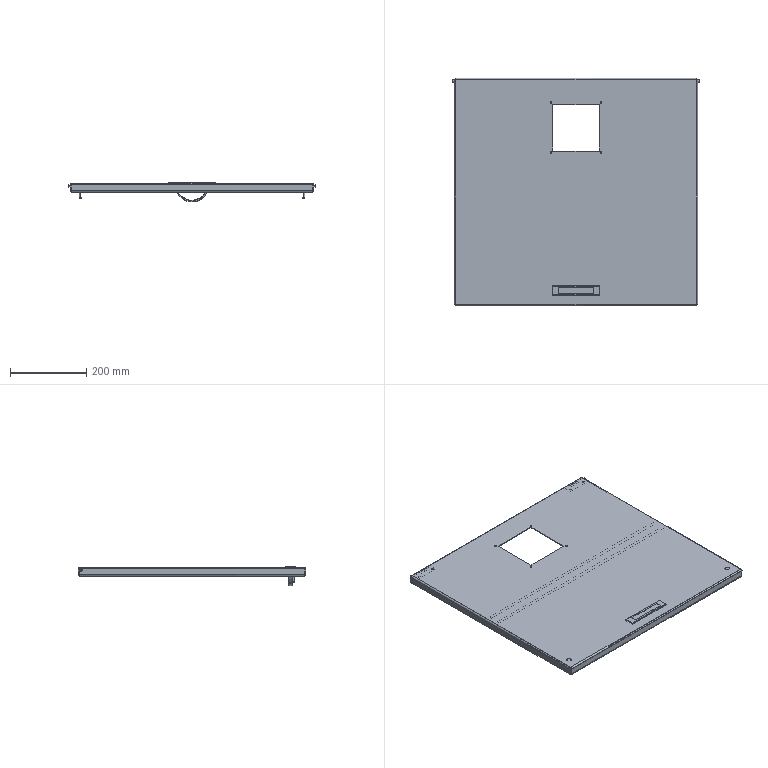Part | NX | features BREP 11 | 12 solids | 446 faces | box 648 x 597 x 52 mm | volume 981887 mm3 | plane 184 | cylinder 132 | torus 94 | cone 20 | spline 16 | commonest cylinder face diameters 6 x20 10 x16 4 x14 7 x12 8 x12 2 x8